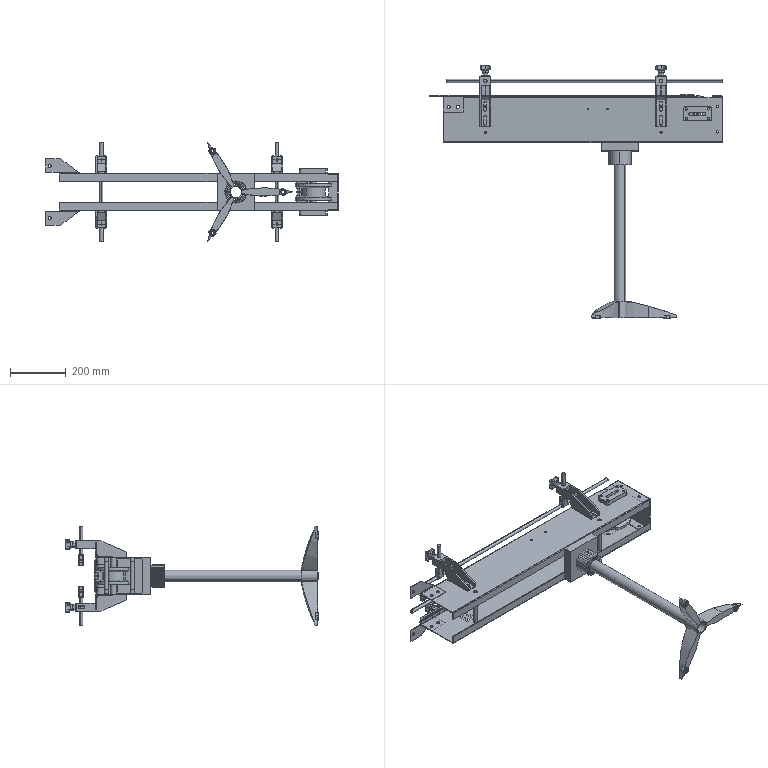Part | SolidWorks | 43 solids | 1465 faces | box 1050 x 909.194 x 355 mm | volume 3666509 mm3 | cylinder 646 | plane 614 | spline 118 | cone 87 | commonest cylinder face diameters 8.5 x80 6 x67 4 x42 1 x40 11 x32 42.2 x32